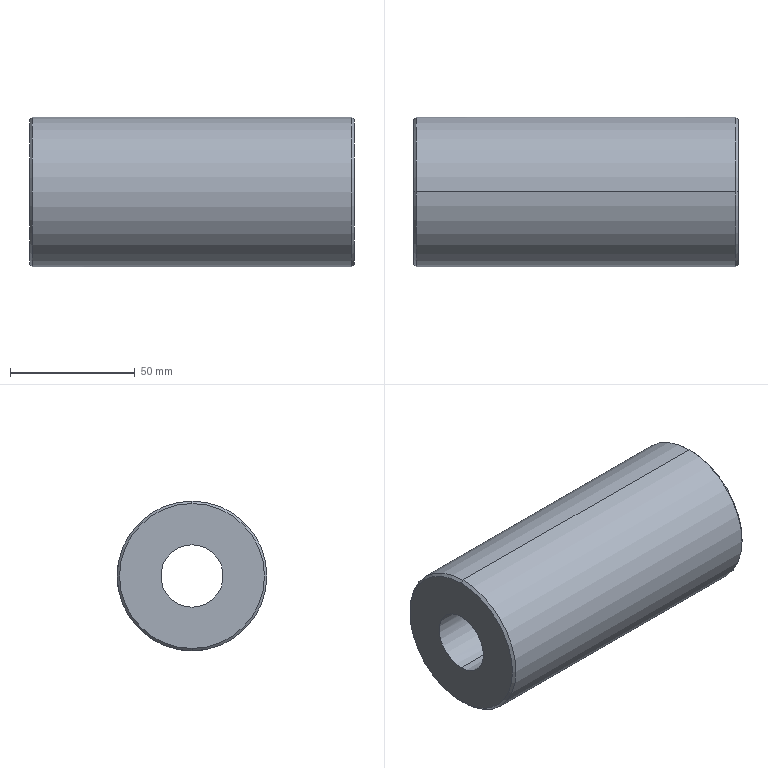Part | STEP file | Sleeve | 1 solid | 18 faces | box 130 x 60 x 60 mm | volume 302189 mm3 | cylinder 12 | cone 4 | plane 2 | commonest cylinder face diameters 5 x8 25 x2 60 x2
STEP:
#1=CARTESIAN_POINT('',(40.,29.896,2.5));
#2=VERTEX_POINT('',#1);
#3=CARTESIAN_POINT('',(40.,29.896,-2.5));
#4=VERTEX_POINT('',#3);
#5=CARTESIAN_POINT('',(40.,29.896,2.5));
#6=CARTESIAN_POINT('',(39.835,29.896,2.5));
#7=CARTESIAN_POINT('',(39.672,29.897,2.484));
#8=CARTESIAN_POINT('',(39.353,29.902,2.42));
#9=CARTESIAN_POINT('',(39.194,29.906,2.372));
#10=CARTESIAN_POINT('',(38.891,29.916,2.247));
#11=CARTESIAN_POINT('',(38.748,29.922,2.17));
#12=CARTESIAN_POINT('',(38.476,29.934,1.989));
#13=CARTESIAN_POINT('',(38.347,29.941,1.883));
#14=CARTESIAN_POINT('',(38.117,29.955,1.652));
#15=CARTESIAN_POINT('',(38.013,29.961,1.527));
#16=CARTESIAN_POINT('',(37.831,29.974,1.253));
#17=CARTESIAN_POINT('',(37.753,29.98,1.108));
#18=CARTESIAN_POINT('',(37.628,29.99,0.8074));
#19=CARTESIAN_POINT('',(37.58,29.993,0.6498));
#20=CARTESIAN_POINT('',(37.516,29.999,0.3271));
#21=CARTESIAN_POINT('',(37.5,30.,0.1648));
#22=CARTESIAN_POINT('',(37.5,30.,-0.1614));
#23=CARTESIAN_POINT('',(37.516,29.999,-0.327));
#24=CARTESIAN_POINT('',(37.58,29.993,-0.6477));
#25=CARTESIAN_POINT('',(37.627,29.99,-0.8036));
#26=CARTESIAN_POINT('',(37.752,29.98,-1.106));
#27=CARTESIAN_POINT('',(37.83,29.974,-1.253));
#28=CARTESIAN_POINT('',(38.011,29.962,-1.524));
#29=CARTESIAN_POINT('',(38.114,29.955,-1.65));
#30=CARTESIAN_POINT('',(38.348,29.941,-1.883));
#31=CARTESIAN_POINT('',(38.474,29.934,-1.987));
#32=CARTESIAN_POINT('',(38.744,29.922,-2.168));
#33=CARTESIAN_POINT('',(38.89,29.916,-2.246));
#34=CARTESIAN_POINT('',(39.193,29.906,-2.372));
#35=CARTESIAN_POINT('',(39.349,29.902,-2.419));
#36=CARTESIAN_POINT('',(39.669,29.897,-2.483));
#37=CARTESIAN_POINT('',(39.835,29.896,-2.5));
#38=CARTESIAN_POINT('',(40.,29.896,-2.5));
#39=B_SPLINE_CURVE_WITH_KNOTS('',3,(#5,#6,#7,#8,#9,#10,#11,#12,#13,#14,#15,#16,#17,#18,#19,#20,#21,#22,#23,#24,#25,#26,#27,#28,#29,#30,#31,#32,#33,#34,#35,#36,#37,#38),.UNSPECIFIED.,.F.,.F.,(4,2,2,2,2,2,2,2,2,2,2,2,2,2,2,2,4),(0.007818,0.008306,0.008795,0.009284,0.009772,0.01026,0.01075,0.01124,0.01173,0.01222,0.0127,0.01319,0.01368,0.01417,0.01466,0.01515,0.01564),.UNSPECIFIED.);
#40=EDGE_CURVE('',#2,#4,#39,.T.);
#41=ORIENTED_EDGE('',*,*,#40,.T.);
#42=CARTESIAN_POINT('',(40.,29.896,-2.5));
#43=CARTESIAN_POINT('',(40.165,29.896,-2.5));
#44=CARTESIAN_POINT('',(40.328,29.897,-2.484));
#45=CARTESIAN_POINT('',(40.647,29.902,-2.42));
#46=CARTESIAN_POINT('',(40.806,29.906,-2.372));
#47=CARTESIAN_POINT('',(41.109,29.916,-2.247));
#48=CARTESIAN_POINT('',(41.252,29.922,-2.17));
#49=CARTESIAN_POINT('',(41.524,29.934,-1.989));
#50=CARTESIAN_POINT('',(41.653,29.941,-1.883));
#51=CARTESIAN_POINT('',(41.883,29.955,-1.652));
#52=CARTESIAN_POINT('',(41.987,29.961,-1.527));
#53=CARTESIAN_POINT('',(42.169,29.974,-1.253));
#54=CARTESIAN_POINT('',(42.247,29.98,-1.108));
#55=CARTESIAN_POINT('',(42.372,29.99,-0.8074));
#56=CARTESIAN_POINT('',(42.42,29.993,-0.6498));
#57=CARTESIAN_POINT('',(42.484,29.999,-0.3271));
#58=CARTESIAN_POINT('',(42.5,30.,-0.1648));
#59=CARTESIAN_POINT('',(42.5,30.,0.1614));
#60=CARTESIAN_POINT('',(42.484,29.999,0.327));
#61=CARTESIAN_POINT('',(42.42,29.993,0.6477));
#62=CARTESIAN_POINT('',(42.373,29.99,0.8036));
#63=CARTESIAN_POINT('',(42.248,29.98,1.106));
#64=CARTESIAN_POINT('',(42.17,29.974,1.253));
#65=CARTESIAN_POINT('',(41.989,29.962,1.524));
#66=CARTESIAN_POINT('',(41.886,29.955,1.65));
#67=CARTESIAN_POINT('',(41.652,29.941,1.883));
#68=CARTESIAN_POINT('',(41.526,29.934,1.987));
#69=CARTESIAN_POINT('',(41.256,29.922,2.168));
#70=CARTESIAN_POINT('',(41.11,29.916,2.246));
#71=CARTESIAN_POINT('',(40.807,29.906,2.372));
#72=CARTESIAN_POINT('',(40.651,29.902,2.419));
#73=CARTESIAN_POINT('',(40.331,29.897,2.483));
#74=CARTESIAN_POINT('',(40.165,29.896,2.5));
#75=CARTESIAN_POINT('',(40.,29.896,2.5));
#76=B_SPLINE_CURVE_WITH_KNOTS('',3,(#42,#43,#44,#45,#46,#47,#48,#49,#50,#51,#52,#53,#54,#55,#56,#57,#58,#59,#60,#61,#62,#63,#64,#65,#66,#67,#68,#69,#70,#71,#72,#73,#74,#75),.UNSPECIFIED.,.F.,.F.,(4,2,2,2,2,2,2,2,2,2,2,2,2,2,2,2,4),(0.,0.0004886,0.0009772,0.001466,0.001954,0.002443,0.002932,0.00342,0.003909,0.004398,0.004886,0.005375,0.005863,0.006352,0.006841,0.007329,0.007818),.UNSPECIFIED.);
#77=EDGE_CURVE('',#4,#2,#76,.T.);
#78=ORIENTED_EDGE('',*,*,#77,.T.);
#79=EDGE_LOOP('',(#41,#78));
#80=FACE_BOUND('',#79,.T.);
#81=CARTESIAN_POINT('',(-40.,29.896,2.5));
#82=VERTEX_POINT('',#81);
#83=CARTESIAN_POINT('',(-40.,29.896,-2.5));
#84=VERTEX_POINT('',#83);
#85=CARTESIAN_POINT('',(-40.,29.896,2.5));
#86=CARTESIAN_POINT('',(-40.165,29.896,2.5));
#87=CARTESIAN_POINT('',(-40.328,29.897,2.484));
#88=CARTESIAN_POINT('',(-40.647,29.902,2.42));
#89=CARTESIAN_POINT('',(-40.806,29.906,2.372));
#90=CARTESIAN_POINT('',(-41.109,29.916,2.247));
#91=CARTESIAN_POINT('',(-41.252,29.922,2.17));
#92=CARTESIAN_POINT('',(-41.524,29.934,1.989));
#93=CARTESIAN_POINT('',(-41.653,29.941,1.883));
#94=CARTESIAN_POINT('',(-41.883,29.955,1.652));
#95=CARTESIAN_POINT('',(-41.987,29.961,1.527));
#96=CARTESIAN_POINT('',(-42.169,29.974,1.253));
#97=CARTESIAN_POINT('',(-42.247,29.98,1.108));
#98=CARTESIAN_POINT('',(-42.372,29.99,0.8074));
#99=CARTESIAN_POINT('',(-42.42,29.993,0.6498));
#100=CARTESIAN_POINT('',(-42.484,29.999,0.3271));
#101=CARTESIAN_POINT('',(-42.5,30.,0.1648));
#102=CARTESIAN_POINT('',(-42.5,30.,-0.1614));
#103=CARTESIAN_POINT('',(-42.484,29.999,-0.327));
#104=CARTESIAN_POINT('',(-42.42,29.993,-0.6477));
#105=CARTESIAN_POINT('',(-42.373,29.99,-0.8036));
#106=CARTESIAN_POINT('',(-42.248,29.98,-1.106));
#107=CARTESIAN_POINT('',(-42.17,29.974,-1.253));
#108=CARTESIAN_POINT('',(-41.989,29.962,-1.524));
#109=CARTESIAN_POINT('',(-41.886,29.955,-1.65));
#110=CARTESIAN_POINT('',(-41.652,29.941,-1.883));
#111=CARTESIAN_POINT('',(-41.526,29.934,-1.987));
#112=CARTESIAN_POINT('',(-41.256,29.922,-2.168));
#113=CARTESIAN_POINT('',(-41.11,29.916,-2.246));
#114=CARTESIAN_POINT('',(-40.807,29.906,-2.372));
#115=CARTESIAN_POINT('',(-40.651,29.902,-2.419));
#116=CARTESIAN_POINT('',(-40.331,29.897,-2.483));
#117=CARTESIAN_POINT('',(-40.165,29.896,-2.5));
#118=CARTESIAN_POINT('',(-40.,29.896,-2.5));
#119=B_SPLINE_CURVE_WITH_KNOTS('',3,(#85,#86,#87,#88,#89,#90,#91,#92,#93,#94,#95,#96,#97,#98,#99,#100,#101,#102,#103,#104,#105,#106,#107,#108,#109,#110,#111,#112,#113,#114,#115,#116,#117,#118),.UNSPECIFIED.,.F.,.F.,(4,2,2,2,2,2,2,2,2,2,2,2,2,2,2,2,4),(0.007818,0.008306,0.008795,0.009284,0.009772,0.01026,0.01075,0.01124,0.01173,0.01222,0.0127,0.01319,0.01368,0.01417,0.01466,0.01515,0.01564),.UNSPECIFIED.);
#120=EDGE_CURVE('',#82,#84,#119,.T.);
#121=ORIENTED_EDGE('',*,*,#120,.T.);
#122=CARTESIAN_POINT('',(-40.,29.896,-2.5));
#123=CARTESIAN_POINT('',(-39.835,29.896,-2.5));
#124=CARTESIAN_POINT('',(-39.672,29.897,-2.484));
#125=CARTESIAN_POINT('',(-39.353,29.902,-2.42));
#126=CARTESIAN_POINT('',(-39.194,29.906,-2.372));
#127=CARTESIAN_POINT('',(-38.891,29.916,-2.247));
#128=CARTESIAN_POINT('',(-38.748,29.922,-2.17));
#129=CARTESIAN_POINT('',(-38.476,29.934,-1.989));
#130=CARTESIAN_POINT('',(-38.347,29.941,-1.883));
#131=CARTESIAN_POINT('',(-38.117,29.955,-1.652));
#132=CARTESIAN_POINT('',(-38.013,29.961,-1.527));
#133=CARTESIAN_POINT('',(-37.831,29.974,-1.253));
#134=CARTESIAN_POINT('',(-37.753,29.98,-1.108));
#135=CARTESIAN_POINT('',(-37.628,29.99,-0.8074));
#136=CARTESIAN_POINT('',(-37.58,29.993,-0.6498));
#137=CARTESIAN_POINT('',(-37.516,29.999,-0.3271));
#138=CARTESIAN_POINT('',(-37.5,30.,-0.1648));
#139=CARTESIAN_POINT('',(-37.5,30.,0.1614));
#140=CARTESIAN_POINT('',(-37.516,29.999,0.327));
#141=CARTESIAN_POINT('',(-37.58,29.993,0.6477));
#142=CARTESIAN_POINT('',(-37.627,29.99,0.8036));
#143=CARTESIAN_POINT('',(-37.752,29.98,1.106));
#144=CARTESIAN_POINT('',(-37.83,29.974,1.253));
#145=CARTESIAN_POINT('',(-38.011,29.962,1.524));
#146=CARTESIAN_POINT('',(-38.114,29.955,1.65));
#147=CARTESIAN_POINT('',(-38.348,29.941,1.883));
#148=CARTESIAN_POINT('',(-38.474,29.934,1.987));
#149=CARTESIAN_POINT('',(-38.744,29.922,2.168));
#150=CARTESIAN_POINT('',(-38.89,29.916,2.246));
#151=CARTESIAN_POINT('',(-39.193,29.906,2.372));
#152=CARTESIAN_POINT('',(-39.349,29.902,2.419));
#153=CARTESIAN_POINT('',(-39.669,29.897,2.483));
#154=CARTESIAN_POINT('',(-39.835,29.896,2.5));
#155=CARTESIAN_POINT('',(-40.,29.896,2.5));
#156=B_SPLINE_CURVE_WITH_KNOTS('',3,(#122,#123,#124,#125,#126,#127,#128,#129,#130,#131,#132,#133,#134,#135,#136,#137,#138,#139,#140,#141,#142,#143,#144,#145,#146,#147,#148,#149,#150,#151,#152,#153,#154,#155),.UNSPECIFIED.,.F.,.F.,(4,2,2,2,2,2,2,2,2,2,2,2,2,2,2,2,4),(0.,0.0004886,0.0009772,0.001466,0.001954,0.002443,0.002932,0.00342,0.003909,0.004398,0.004886,0.005375,0.005863,0.006352,0.006841,0.007329,0.007818),.UNSPECIFIED.);
#157=EDGE_CURVE('',#84,#82,#156,.T.);
#158=ORIENTED_EDGE('',*,*,#157,.T.);
#159=EDGE_LOOP('',(#121,#158));
#160=FACE_BOUND('',#159,.T.);
#161=CARTESIAN_POINT('',(64.,0.,30.));
#162=VERTEX_POINT('',#161);
#163=CARTESIAN_POINT('',(64.,0.,-30.));
#164=VERTEX_POINT('',#163);
#165=CARTESIAN_POINT('',(64.,0.,0.));
#166=DIRECTION('',(-1.,0.,0.));
#167=DIRECTION('',(0.,0.,1.));
#168=AXIS2_PLACEMENT_3D('',#165,#166,#167);
#169=CIRCLE('',#168,30.);
#170=EDGE_CURVE('',#162,#164,#169,.T.);
#171=ORIENTED_EDGE('',*,*,#170,.T.);
#172=CARTESIAN_POINT('',(42.5,0.,-30.));
#173=VERTEX_POINT('',#172);
#174=CARTESIAN_POINT('',(65.,0.,-30.));
#175=DIRECTION('',(-1.,0.,0.));
#176=VECTOR('',#175,1000.);
#177=LINE('',#174,#176);
#178=EDGE_CURVE('',#164,#173,#177,.T.);
#179=ORIENTED_EDGE('',*,*,#178,.T.);
#180=CARTESIAN_POINT('',(40.,2.5,-29.896));
#181=VERTEX_POINT('',#180);
#182=CARTESIAN_POINT('',(42.5,0.,-30.));
#183=CARTESIAN_POINT('',(42.5,0.1651,-30.));
#184=CARTESIAN_POINT('',(42.484,0.3275,-29.999));
#185=CARTESIAN_POINT('',(42.42,0.6469,-29.993));
#186=CARTESIAN_POINT('',(42.372,0.8057,-29.99));
#187=CARTESIAN_POINT('',(42.247,1.108,-29.98));
#188=CARTESIAN_POINT('',(42.17,1.252,-29.974));
#189=CARTESIAN_POINT('',(41.989,1.523,-29.962));
#190=CARTESIAN_POINT('',(41.884,1.652,-29.955));
#191=CARTESIAN_POINT('',(41.653,1.882,-29.941));
#192=CARTESIAN_POINT('',(41.528,1.986,-29.934));
#193=CARTESIAN_POINT('',(41.255,2.169,-29.922));
#194=CARTESIAN_POINT('',(41.109,2.246,-29.916));
#195=CARTESIAN_POINT('',(40.658,2.434,-29.901));
#196=CARTESIAN_POINT('',(40.33,2.5,-29.896));
#197=CARTESIAN_POINT('',(40.,2.5,-29.896));
#198=B_SPLINE_CURVE_WITH_KNOTS('',3,(#182,#183,#184,#185,#186,#187,#188,#189,#190,#191,#192,#193,#194,#195,#196,#197),.UNSPECIFIED.,.F.,.F.,(4,2,2,2,2,2,2,4),(0.007814,0.008303,0.008791,0.009279,0.009768,0.01026,0.01074,0.01172),.UNSPECIFIED.);
#199=EDGE_CURVE('',#173,#181,#198,.T.);
#200=ORIENTED_EDGE('',*,*,#199,.T.);
#201=CARTESIAN_POINT('',(37.5,0.,-30.));
#202=VERTEX_POINT('',#201);
#203=CARTESIAN_POINT('',(40.,2.5,-29.896));
#204=CARTESIAN_POINT('',(39.835,2.5,-29.896));
#205=CARTESIAN_POINT('',(39.672,2.484,-29.897));
#206=CARTESIAN_POINT('',(39.353,2.42,-29.902));
#207=CARTESIAN_POINT('',(39.194,2.372,-29.906));
#208=CARTESIAN_POINT('',(38.892,2.247,-29.916));
#209=CARTESIAN_POINT('',(38.748,2.17,-29.922));
#210=CARTESIAN_POINT('',(38.477,1.989,-29.934));
#211=CARTESIAN_POINT('',(38.348,1.884,-29.941));
#212=CARTESIAN_POINT('',(38.118,1.653,-29.955));
#213=CARTESIAN_POINT('',(38.014,1.528,-29.961));
#214=CARTESIAN_POINT('',(37.831,1.255,-29.974));
#215=CARTESIAN_POINT('',(37.754,1.109,-29.98));
#216=CARTESIAN_POINT('',(37.566,0.6585,-29.994));
#217=CARTESIAN_POINT('',(37.5,0.3303,-30.));
#218=CARTESIAN_POINT('',(37.5,0.,-30.));
#219=B_SPLINE_CURVE_WITH_KNOTS('',3,(#203,#204,#205,#206,#207,#208,#209,#210,#211,#212,#213,#214,#215,#216,#217,#218),.UNSPECIFIED.,.F.,.F.,(4,2,2,2,2,2,2,4),(-0.003907,-0.003419,-0.00293,-0.002442,-0.001954,-0.001465,-0.0009768,0.),.UNSPECIFIED.);
#220=EDGE_CURVE('',#181,#202,#219,.T.);
#221=ORIENTED_EDGE('',*,*,#220,.T.);
#222=CARTESIAN_POINT('',(-37.5,0.,-30.));
#223=VERTEX_POINT('',#222);
#224=CARTESIAN_POINT('',(65.,0.,-30.));
#225=DIRECTION('',(-1.,0.,0.));
#226=VECTOR('',#225,1000.);
#227=LINE('',#224,#226);
#228=EDGE_CURVE('',#202,#223,#227,.T.);
#229=ORIENTED_EDGE('',*,*,#228,.T.);
#230=CARTESIAN_POINT('',(-40.,2.5,-29.896));
#231=VERTEX_POINT('',#230);
#232=CARTESIAN_POINT('',(-37.5,0.,-30.));
#233=CARTESIAN_POINT('',(-37.5,0.1651,-30.));
#234=CARTESIAN_POINT('',(-37.516,0.3275,-29.999));
#235=CARTESIAN_POINT('',(-37.58,0.6469,-29.993));
#236=CARTESIAN_POINT('',(-37.628,0.8057,-29.99));
#237=CARTESIAN_POINT('',(-37.753,1.108,-29.98));
#238=CARTESIAN_POINT('',(-37.83,1.252,-29.974));
#239=CARTESIAN_POINT('',(-38.011,1.523,-29.962));
#240=CARTESIAN_POINT('',(-38.116,1.652,-29.955));
#241=CARTESIAN_POINT('',(-38.347,1.882,-29.941));
#242=CARTESIAN_POINT('',(-38.472,1.986,-29.934));
#243=CARTESIAN_POINT('',(-38.745,2.169,-29.922));
#244=CARTESIAN_POINT('',(-38.891,2.246,-29.916));
#245=CARTESIAN_POINT('',(-39.342,2.434,-29.901));
#246=CARTESIAN_POINT('',(-39.67,2.5,-29.896));
#247=CARTESIAN_POINT('',(-40.,2.5,-29.896));
#248=B_SPLINE_CURVE_WITH_KNOTS('',3,(#232,#233,#234,#235,#236,#237,#238,#239,#240,#241,#242,#243,#244,#245,#246,#247),.UNSPECIFIED.,.F.,.F.,(4,2,2,2,2,2,2,4),(0.007814,0.008303,0.008791,0.009279,0.009768,0.01026,0.01074,0.01172),.UNSPECIFIED.);
#249=EDGE_CURVE('',#223,#231,#248,.T.);
#250=ORIENTED_EDGE('',*,*,#249,.T.);
#251=CARTESIAN_POINT('',(-42.5,0.,-30.));
#252=VERTEX_POINT('',#251);
#253=CARTESIAN_POINT('',(-40.,2.5,-29.896));
#254=CARTESIAN_POINT('',(-40.165,2.5,-29.896));
#255=CARTESIAN_POINT('',(-40.328,2.484,-29.897));
#256=CARTESIAN_POINT('',(-40.647,2.42,-29.902));
#257=CARTESIAN_POINT('',(-40.806,2.372,-29.906));
#258=CARTESIAN_POINT('',(-41.108,2.247,-29.916));
#259=CARTESIAN_POINT('',(-41.252,2.17,-29.922));
#260=CARTESIAN_POINT('',(-41.523,1.989,-29.934));
#261=CARTESIAN_POINT('',(-41.652,1.884,-29.941));
#262=CARTESIAN_POINT('',(-41.882,1.653,-29.955));
#263=CARTESIAN_POINT('',(-41.986,1.528,-29.961));
#264=CARTESIAN_POINT('',(-42.169,1.255,-29.974));
#265=CARTESIAN_POINT('',(-42.246,1.109,-29.98));
#266=CARTESIAN_POINT('',(-42.434,0.6585,-29.994));
#267=CARTESIAN_POINT('',(-42.5,0.3303,-30.));
#268=CARTESIAN_POINT('',(-42.5,0.,-30.));
#269=B_SPLINE_CURVE_WITH_KNOTS('',3,(#253,#254,#255,#256,#257,#258,#259,#260,#261,#262,#263,#264,#265,#266,#267,#268),.UNSPECIFIED.,.F.,.F.,(4,2,2,2,2,2,2,4),(0.01172,0.01221,0.0127,0.01319,0.01367,0.01416,0.01465,0.01563),.UNSPECIFIED.);
#270=EDGE_CURVE('',#231,#252,#269,.T.);
#271=ORIENTED_EDGE('',*,*,#270,.T.);
#272=CARTESIAN_POINT('',(-64.,0.,-30.));
#273=VERTEX_POINT('',#272);
#274=CARTESIAN_POINT('',(65.,0.,-30.));
#275=DIRECTION('',(-1.,0.,0.));
#276=VECTOR('',#275,1000.);
#277=LINE('',#274,#276);
#278=EDGE_CURVE('',#252,#273,#277,.T.);
#279=ORIENTED_EDGE('',*,*,#278,.T.);
#280=CARTESIAN_POINT('',(-64.,0.,30.));
#281=VERTEX_POINT('',#280);
#282=CARTESIAN_POINT('',(-64.,0.,0.));
#283=DIRECTION('',(1.,0.,0.));
#284=DIRECTION('',(0.,0.,1.));
#285=AXIS2_PLACEMENT_3D('',#282,#283,#284);
#286=CIRCLE('',#285,30.);
#287=EDGE_CURVE('',#273,#281,#286,.T.);
#288=ORIENTED_EDGE('',*,*,#287,.T.);
#289=CARTESIAN_POINT('',(65.,0.,30.));
#290=DIRECTION('',(-1.,0.,0.));
#291=VECTOR('',#290,1000.);
#292=LINE('',#289,#291);
#293=EDGE_CURVE('',#162,#281,#292,.T.);
#294=ORIENTED_EDGE('',*,*,#293,.F.);
#295=EDGE_LOOP('',(#171,#179,#200,#221,#229,#250,#271,#279,#288,#294));
#296=FACE_OUTER_BOUND('',#295,.T.);
#297=CARTESIAN_POINT('',(65.,0.,0.));
#298=DIRECTION('',(-1.,0.,0.));
#299=DIRECTION('',(0.,0.,1.));
#300=AXIS2_PLACEMENT_3D('',#297,#298,#299);
#301=CYLINDRICAL_SURFACE('',#300,30.);
#302=ADVANCED_FACE('',(#80,#160,#296),#301,.T.);
#303=CARTESIAN_POINT('',(40.,-2.5,-12.247));
#304=VERTEX_POINT('',#303);
#305=CARTESIAN_POINT('',(37.5,0.,-12.5));
#306=VERTEX_POINT('',#305);
#307=CARTESIAN_POINT('',(40.,-2.5,-12.247));
#308=CARTESIAN_POINT('',(39.834,-2.5,-12.247));
#309=CARTESIAN_POINT('',(39.672,-2.484,-12.251));
#310=CARTESIAN_POINT('',(39.352,-2.42,-12.264));
#311=CARTESIAN_POINT('',(39.193,-2.372,-12.273));
#312=CARTESIAN_POINT('',(38.891,-2.246,-12.297));
#313=CARTESIAN_POINT('',(38.747,-2.17,-12.311));
#314=CARTESIAN_POINT('',(38.476,-1.988,-12.341));
#315=CARTESIAN_POINT('',(38.348,-1.883,-12.358));
#316=CARTESIAN_POINT('',(38.003,-1.539,-12.407));
#317=CARTESIAN_POINT('',(37.817,-1.261,-12.44));
#318=CARTESIAN_POINT('',(37.567,-0.6598,-12.486));
#319=CARTESIAN_POINT('',(37.5,-0.331,-12.5));
#320=CARTESIAN_POINT('',(37.5,0.,-12.5));
#321=B_SPLINE_CURVE_WITH_KNOTS('',3,(#307,#308,#309,#310,#311,#312,#313,#314,#315,#316,#317,#318,#319,#320),.UNSPECIFIED.,.F.,.F.,(4,2,2,2,2,2,4),(0.003915,0.004405,0.004894,0.005384,0.005873,0.006852,0.007831),.UNSPECIFIED.);
#322=EDGE_CURVE('',#304,#306,#321,.T.);
#323=ORIENTED_EDGE('',*,*,#322,.F.);
#324=CARTESIAN_POINT('',(40.,-2.5,-29.896));
#325=VERTEX_POINT('',#324);
#326=CARTESIAN_POINT('',(40.,-2.5,-30.));
#327=DIRECTION('',(0.,0.,-1.));
#328=VECTOR('',#327,1000.);
#329=LINE('',#326,#328);
#330=EDGE_CURVE('',#304,#325,#329,.T.);
#331=ORIENTED_EDGE('',*,*,#330,.T.);
#332=CARTESIAN_POINT('',(37.5,0.,-30.));
#333=CARTESIAN_POINT('',(37.5,-0.1651,-30.));
#334=CARTESIAN_POINT('',(37.516,-0.3275,-29.999));
#335=CARTESIAN_POINT('',(37.58,-0.6469,-29.993));
#336=CARTESIAN_POINT('',(37.628,-0.8057,-29.99));
#337=CARTESIAN_POINT('',(37.753,-1.108,-29.98));
#338=CARTESIAN_POINT('',(37.83,-1.252,-29.974));
#339=CARTESIAN_POINT('',(38.011,-1.523,-29.962));
#340=CARTESIAN_POINT('',(38.116,-1.652,-29.955));
#341=CARTESIAN_POINT('',(38.347,-1.882,-29.941));
#342=CARTESIAN_POINT('',(38.472,-1.986,-29.934));
#343=CARTESIAN_POINT('',(38.745,-2.169,-29.922));
#344=CARTESIAN_POINT('',(38.891,-2.246,-29.916));
#345=CARTESIAN_POINT('',(39.342,-2.434,-29.901));
#346=CARTESIAN_POINT('',(39.67,-2.5,-29.896));
#347=CARTESIAN_POINT('',(40.,-2.5,-29.896));
#348=B_SPLINE_CURVE_WITH_KNOTS('',3,(#332,#333,#334,#335,#336,#337,#338,#339,#340,#341,#342,#343,#344,#345,#346,#347),.UNSPECIFIED.,.F.,.F.,(4,2,2,2,2,2,2,4),(0.,0.0004884,0.0009768,0.001465,0.001954,0.002442,0.00293,0.003907),.UNSPECIFIED.);
#349=EDGE_CURVE('',#202,#325,#348,.T.);
#350=ORIENTED_EDGE('',*,*,#349,.F.);
#351=ORIENTED_EDGE('',*,*,#220,.F.);
#352=CARTESIAN_POINT('',(40.,2.5,-12.247));
#353=VERTEX_POINT('',#352);
#354=CARTESIAN_POINT('',(40.,2.5,-30.));
#355=DIRECTION('',(0.,0.,-1.));
#356=VECTOR('',#355,1000.);
#357=LINE('',#354,#356);
#358=EDGE_CURVE('',#353,#181,#357,.T.);
#359=ORIENTED_EDGE('',*,*,#358,.F.);
#360=CARTESIAN_POINT('',(37.5,0.,-12.5));
#361=CARTESIAN_POINT('',(37.5,0.1655,-12.5));
#362=CARTESIAN_POINT('',(37.516,0.3282,-12.497));
#363=CARTESIAN_POINT('',(37.58,0.6481,-12.484));
#364=CARTESIAN_POINT('',(37.628,0.807,-12.475));
#365=CARTESIAN_POINT('',(37.754,1.109,-12.452));
#366=CARTESIAN_POINT('',(37.83,1.253,-12.438));
#367=CARTESIAN_POINT('',(38.012,1.524,-12.407));
#368=CARTESIAN_POINT('',(38.117,1.652,-12.391));
#369=CARTESIAN_POINT('',(38.462,1.997,-12.342));
#370=CARTESIAN_POINT('',(38.739,2.183,-12.309));
#371=CARTESIAN_POINT('',(39.34,2.433,-12.262));
#372=CARTESIAN_POINT('',(39.669,2.5,-12.247));
#373=CARTESIAN_POINT('',(40.,2.5,-12.247));
#374=B_SPLINE_CURVE_WITH_KNOTS('',3,(#360,#361,#362,#363,#364,#365,#366,#367,#368,#369,#370,#371,#372,#373),.UNSPECIFIED.,.F.,.F.,(4,2,2,2,2,2,4),(0.007831,0.00832,0.00881,0.009299,0.009788,0.01077,0.01175),.UNSPECIFIED.);
#375=EDGE_CURVE('',#306,#353,#374,.T.);
#376=ORIENTED_EDGE('',*,*,#375,.F.);
#377=EDGE_LOOP('',(#323,#331,#350,#351,#359,#376));
#378=FACE_OUTER_BOUND('',#377,.T.);
#379=CARTESIAN_POINT('',(40.,0.,-30.));
#380=DIRECTION('',(0.,0.,-1.));
#381=DIRECTION('',(0.,1.,0.));
#382=AXIS2_PLACEMENT_3D('',#379,#380,#381);
#383=CYLINDRICAL_SURFACE('',#382,2.5);
#384=ADVANCED_FACE('',(#378),#383,.F.);
#385=CARTESIAN_POINT('',(-40.,-2.5,-12.247));
#386=VERTEX_POINT('',#385);
#387=CARTESIAN_POINT('',(-42.5,0.,-12.5));
#388=VERTEX_POINT('',#387);
#389=CARTESIAN_POINT('',(-40.,-2.5,-12.247));
#390=CARTESIAN_POINT('',(-40.166,-2.5,-12.247));
#391=CARTESIAN_POINT('',(-40.328,-2.484,-12.251));
#392=CARTESIAN_POINT('',(-40.648,-2.42,-12.264));
#393=CARTESIAN_POINT('',(-40.807,-2.372,-12.273));
#394=CARTESIAN_POINT('',(-41.109,-2.246,-12.297));
#395=CARTESIAN_POINT('',(-41.253,-2.17,-12.311));
#396=CARTESIAN_POINT('',(-41.524,-1.988,-12.341));
#397=CARTESIAN_POINT('',(-41.652,-1.883,-12.358));
#398=CARTESIAN_POINT('',(-41.997,-1.539,-12.407));
#399=CARTESIAN_POINT('',(-42.183,-1.261,-12.44));
#400=CARTESIAN_POINT('',(-42.433,-0.6598,-12.486));
#401=CARTESIAN_POINT('',(-42.5,-0.331,-12.5));
#402=CARTESIAN_POINT('',(-42.5,0.,-12.5));
#403=B_SPLINE_CURVE_WITH_KNOTS('',3,(#389,#390,#391,#392,#393,#394,#395,#396,#397,#398,#399,#400,#401,#402),.UNSPECIFIED.,.F.,.F.,(4,2,2,2,2,2,4),(0.003915,0.004405,0.004894,0.005384,0.005873,0.006852,0.007831),.UNSPECIFIED.);
#404=EDGE_CURVE('',#386,#388,#403,.T.);
#405=ORIENTED_EDGE('',*,*,#404,.F.);
#406=CARTESIAN_POINT('',(-40.,-2.5,-29.896));
#407=VERTEX_POINT('',#406);
#408=CARTESIAN_POINT('',(-40.,-2.5,-30.));
#409=DIRECTION('',(0.,0.,-1.));
#410=VECTOR('',#409,1000.);
#411=LINE('',#408,#410);
#412=EDGE_CURVE('',#386,#407,#411,.T.);
#413=ORIENTED_EDGE('',*,*,#412,.T.);
#414=CARTESIAN_POINT('',(-42.5,0.,-30.));
#415=CARTESIAN_POINT('',(-42.5,-0.1651,-30.));
#416=CARTESIAN_POINT('',(-42.484,-0.3275,-29.999));
#417=CARTESIAN_POINT('',(-42.42,-0.6469,-29.993));
#418=CARTESIAN_POINT('',(-42.372,-0.8057,-29.99));
#419=CARTESIAN_POINT('',(-42.247,-1.108,-29.98));
#420=CARTESIAN_POINT('',(-42.17,-1.252,-29.974));
#421=CARTESIAN_POINT('',(-41.989,-1.523,-29.962));
#422=CARTESIAN_POINT('',(-41.884,-1.652,-29.955));
#423=CARTESIAN_POINT('',(-41.653,-1.882,-29.941));
#424=CARTESIAN_POINT('',(-41.528,-1.986,-29.934));
#425=CARTESIAN_POINT('',(-41.255,-2.169,-29.922));
#426=CARTESIAN_POINT('',(-41.109,-2.246,-29.916));
#427=CARTESIAN_POINT('',(-40.658,-2.434,-29.901));
#428=CARTESIAN_POINT('',(-40.33,-2.5,-29.896));
#429=CARTESIAN_POINT('',(-40.,-2.5,-29.896));
#430=B_SPLINE_CURVE_WITH_KNOTS('',3,(#414,#415,#416,#417,#418,#419,#420,#421,#422,#423,#424,#425,#426,#427,#428,#429),.UNSPECIFIED.,.F.,.F.,(4,2,2,2,2,2,2,4),(0.,0.0004884,0.0009768,0.001465,0.001954,0.002442,0.00293,0.003907),.UNSPECIFIED.);
#431=EDGE_CURVE('',#252,#407,#430,.T.);
#432=ORIENTED_EDGE('',*,*,#431,.F.);
#433=ORIENTED_EDGE('',*,*,#270,.F.);
#434=CARTESIAN_POINT('',(-40.,2.5,-12.247));
#435=VERTEX_POINT('',#434);
#436=CARTESIAN_POINT('',(-40.,2.5,-30.));
#437=DIRECTION('',(0.,0.,-1.));
#438=VECTOR('',#437,1000.);
#439=LINE('',#436,#438);
#440=EDGE_CURVE('',#435,#231,#439,.T.);
#441=ORIENTED_EDGE('',*,*,#440,.F.);
#442=CARTESIAN_POINT('',(-42.5,0.,-12.5));
#443=CARTESIAN_POINT('',(-42.5,0.1655,-12.5));
#444=CARTESIAN_POINT('',(-42.484,0.3282,-12.497));
#445=CARTESIAN_POINT('',(-42.42,0.6481,-12.484));
#446=CARTESIAN_POINT('',(-42.372,0.807,-12.475));
#447=CARTESIAN_POINT('',(-42.246,1.109,-12.452));
#448=CARTESIAN_POINT('',(-42.17,1.253,-12.438));
#449=CARTESIAN_POINT('',(-41.988,1.524,-12.407));
#450=CARTESIAN_POINT('',(-41.883,1.652,-12.391));
#451=CARTESIAN_POINT('',(-41.538,1.997,-12.342));
#452=CARTESIAN_POINT('',(-41.261,2.183,-12.309));
#453=CARTESIAN_POINT('',(-40.66,2.433,-12.262));
#454=CARTESIAN_POINT('',(-40.331,2.5,-12.247));
#455=CARTESIAN_POINT('',(-40.,2.5,-12.247));
#456=B_SPLINE_CURVE_WITH_KNOTS('',3,(#442,#443,#444,#445,#446,#447,#448,#449,#450,#451,#452,#453,#454,#455),.UNSPECIFIED.,.F.,.F.,(4,2,2,2,2,2,4),(0.007831,0.00832,0.00881,0.009299,0.009788,0.01077,0.01175),.UNSPECIFIED.);
#457=EDGE_CURVE('',#388,#435,#456,.T.);
#458=ORIENTED_EDGE('',*,*,#457,.F.);
#459=EDGE_LOOP('',(#405,#413,#432,#433,#441,#458));
#460=FACE_OUTER_BOUND('',#459,.T.);
#461=CARTESIAN_POINT('',(-40.,0.,-30.));
#462=DIRECTION('',(0.,0.,-1.));
#463=DIRECTION('',(0.,1.,0.));
#464=AXIS2_PLACEMENT_3D('',#461,#462,#463);
#465=CYLINDRICAL_SURFACE('',#464,2.5);
#466=ADVANCED_FACE('',(#460),#465,.F.);
#467=CARTESIAN_POINT('',(-65.,0.,-29.));
#468=VERTEX_POINT('',#467);
#469=CARTESIAN_POINT('',(-65.,0.,29.));
#470=VERTEX_POINT('',#469);
#471=CARTESIAN_POINT('',(-65.,0.,0.));
#472=DIRECTION('',(1.,0.,0.));
#473=DIRECTION('',(0.,0.,-1.));
#474=AXIS2_PLACEMENT_3D('',#471,#472,#473);
#475=CIRCLE('',#474,29.);
#476=EDGE_CURVE('',#468,#470,#475,.T.);
#477=ORIENTED_EDGE('',*,*,#476,.T.);
#478=CARTESIAN_POINT('',(-64.,0.,30.));
#479=DIRECTION('',(0.7071,0.,0.7071));
#480=VECTOR('',#479,1000.);
#481=LINE('',#478,#480);
#482=EDGE_CURVE('',#470,#281,#481,.T.);
#483=ORIENTED_EDGE('',*,*,#482,.T.);
#484=ORIENTED_EDGE('',*,*,#287,.F.);
#485=CARTESIAN_POINT('',(-64.,0.,-30.));
#486=DIRECTION('',(0.7071,0.,-0.7071));
#487=VECTOR('',#486,1000.);
#488=LINE('',#485,#487);
#489=EDGE_CURVE('',#468,#273,#488,.T.);
#490=ORIENTED_EDGE('',*,*,#489,.F.);
#491=EDGE_LOOP('',(#477,#483,#484,#490));
#492=FACE_OUTER_BOUND('',#491,.T.);
#493=CARTESIAN_POINT('',(-64.,0.,0.));
#494=DIRECTION('',(1.,0.,0.));
#495=DIRECTION('',(0.,0.,-1.));
#496=AXIS2_PLACEMENT_3D('',#493,#494,#495);
#497=CONICAL_SURFACE('',#496,30.,0.7854);
#498=ADVANCED_FACE('',(#492),#497,.T.);
#499=CARTESIAN_POINT('',(65.,0.,29.));
#500=VERTEX_POINT('',#499);
#501=CARTESIAN_POINT('',(65.,0.,-29.));
#502=VERTEX_POINT('',#501);
#503=CARTESIAN_POINT('',(65.,0.,0.));
#504=DIRECTION('',(-1.,0.,0.));
#505=DIRECTION('',(0.,0.,1.));
#506=AXIS2_PLACEMENT_3D('',#503,#504,#505);
#507=CIRCLE('',#506,29.);
#508=EDGE_CURVE('',#500,#502,#507,.T.);
#509=ORIENTED_EDGE('',*,*,#508,.T.);
#510=CARTESIAN_POINT('',(64.,0.,-30.));
#511=DIRECTION('',(-0.7071,0.,-0.7071));
#512=VECTOR('',#511,1000.);
#513=LINE('',#510,#512);
#514=EDGE_CURVE('',#502,#164,#513,.T.);
#515=ORIENTED_EDGE('',*,*,#514,.T.);
#516=ORIENTED_EDGE('',*,*,#170,.F.);
#517=CARTESIAN_POINT('',(64.,0.,30.));
#518=DIRECTION('',(-0.7071,0.,0.7071));
#519=VECTOR('',#518,1000.);
#520=LINE('',#517,#519);
#521=EDGE_CURVE('',#500,#162,#520,.T.);
#522=ORIENTED_EDGE('',*,*,#521,.F.);
#523=EDGE_LOOP('',(#509,#515,#516,#522));
#524=FACE_OUTER_BOUND('',#523,.T.);
#525=CARTESIAN_POINT('',(64.,0.,0.));
#526=DIRECTION('',(-1.,0.,0.));
#527=DIRECTION('',(0.,0.,1.));
#528=AXIS2_PLACEMENT_3D('',#525,#526,#527);
#529=CONICAL_SURFACE('',#528,30.,0.7854);
#530=ADVANCED_FACE('',(#524),#529,.T.);
#531=CARTESIAN_POINT('',(65.,0.,-12.5));
#532=VERTEX_POINT('',#531);
#533=CARTESIAN_POINT('',(65.,0.,12.5));
#534=VERTEX_POINT('',#533);
#535=CARTESIAN_POINT('',(65.,0.,0.));
#536=DIRECTION('',(-1.,0.,0.));
#537=DIRECTION('',(0.,0.,1.));
#538=AXIS2_PLACEMENT_3D('',#535,#536,#537);
#539=CIRCLE('',#538,12.5);
#540=EDGE_CURVE('',#532,#534,#539,.T.);
#541=ORIENTED_EDGE('',*,*,#540,.F.);
#542=CARTESIAN_POINT('',(42.5,0.,-12.5));
#543=VERTEX_POINT('',#542);
#544=CARTESIAN_POINT('',(65.,0.,-12.5));
#545=DIRECTION('',(-1.,0.,0.));
#546=VECTOR('',#545,1000.);
#547=LINE('',#544,#546);
#548=EDGE_CURVE('',#532,#543,#547,.T.);
#549=ORIENTED_EDGE('',*,*,#548,.T.);
#550=CARTESIAN_POINT('',(42.5,0.,-12.5));
#551=CARTESIAN_POINT('',(42.5,-0.1655,-12.5));
#552=CARTESIAN_POINT('',(42.484,-0.3282,-12.497));
#553=CARTESIAN_POINT('',(42.42,-0.6481,-12.484));
#554=CARTESIAN_POINT('',(42.372,-0.807,-12.475));
#555=CARTESIAN_POINT('',(42.246,-1.109,-12.452));
#556=CARTESIAN_POINT('',(42.17,-1.253,-12.438));
#557=CARTESIAN_POINT('',(41.988,-1.524,-12.407));
#558=CARTESIAN_POINT('',(41.883,-1.652,-12.391));
#559=CARTESIAN_POINT('',(41.538,-1.997,-12.342));
#560=CARTESIAN_POINT('',(41.261,-2.183,-12.309));
#561=CARTESIAN_POINT('',(40.66,-2.433,-12.262));
#562=CARTESIAN_POINT('',(40.331,-2.5,-12.247));
#563=CARTESIAN_POINT('',(40.,-2.5,-12.247));
#564=B_SPLINE_CURVE_WITH_KNOTS('',3,(#550,#551,#552,#553,#554,#555,#556,#557,#558,#559,#560,#561,#562,#563),.UNSPECIFIED.,.F.,.F.,(4,2,2,2,2,2,4),(0.,0.0004894,0.0009788,0.001468,0.001958,0.002936,0.003915),.UNSPECIFIED.);
#565=EDGE_CURVE('',#543,#304,#564,.T.);
#566=ORIENTED_EDGE('',*,*,#565,.T.);
#567=ORIENTED_EDGE('',*,*,#322,.T.);
#568=CARTESIAN_POINT('',(-37.5,0.,-12.5));
#569=VERTEX_POINT('',#568);
#570=CARTESIAN_POINT('',(65.,0.,-12.5));
#571=DIRECTION('',(-1.,0.,0.));
#572=VECTOR('',#571,1000.);
#573=LINE('',#570,#572);
#574=EDGE_CURVE('',#306,#569,#573,.T.);
#575=ORIENTED_EDGE('',*,*,#574,.T.);
#576=CARTESIAN_POINT('',(-37.5,0.,-12.5));
#577=CARTESIAN_POINT('',(-37.5,-0.1655,-12.5));
#578=CARTESIAN_POINT('',(-37.516,-0.3282,-12.497));
#579=CARTESIAN_POINT('',(-37.58,-0.6481,-12.484));
#580=CARTESIAN_POINT('',(-37.628,-0.807,-12.475));
#581=CARTESIAN_POINT('',(-37.754,-1.109,-12.452));
#582=CARTESIAN_POINT('',(-37.83,-1.253,-12.438));
#583=CARTESIAN_POINT('',(-38.012,-1.524,-12.407));
#584=CARTESIAN_POINT('',(-38.117,-1.652,-12.391));
#585=CARTESIAN_POINT('',(-38.462,-1.997,-12.342));
#586=CARTESIAN_POINT('',(-38.739,-2.183,-12.309));
#587=CARTESIAN_POINT('',(-39.34,-2.433,-12.262));
#588=CARTESIAN_POINT('',(-39.669,-2.5,-12.247));
#589=CARTESIAN_POINT('',(-40.,-2.5,-12.247));
#590=B_SPLINE_CURVE_WITH_KNOTS('',3,(#576,#577,#578,#579,#580,#581,#582,#583,#584,#585,#586,#587,#588,#589),.UNSPECIFIED.,.F.,.F.,(4,2,2,2,2,2,4),(0.,0.0004894,0.0009788,0.001468,0.001958,0.002936,0.003915),.UNSPECIFIED.);
#591=EDGE_CURVE('',#569,#386,#590,.T.);
#592=ORIENTED_EDGE('',*,*,#591,.T.);
#593=ORIENTED_EDGE('',*,*,#404,.T.);
#594=CARTESIAN_POINT('',(-65.,0.,-12.5));
#595=VERTEX_POINT('',#594);
#596=CARTESIAN_POINT('',(65.,0.,-12.5));
#597=DIRECTION('',(-1.,0.,0.));
#598=VECTOR('',#597,1000.);
#599=LINE('',#596,#598);
#600=EDGE_CURVE('',#388,#595,#599,.T.);
#601=ORIENTED_EDGE('',*,*,#600,.T.);
#602=CARTESIAN_POINT('',(-65.,0.,12.5));
#603=VERTEX_POINT('',#602);
#604=CARTESIAN_POINT('',(-65.,0.,0.));
#605=DIRECTION('',(1.,0.,0.));
#606=DIRECTION('',(0.,0.,1.));
#607=AXIS2_PLACEMENT_3D('',#604,#605,#606);
#608=CIRCLE('',#607,12.5);
#609=EDGE_CURVE('',#603,#595,#608,.T.);
#610=ORIENTED_EDGE('',*,*,#609,.F.);
#611=CARTESIAN_POINT('',(65.,0.,12.5));
#612=DIRECTION('',(-1.,0.,0.));
#613=VECTOR('',#612,1000.);
#614=LINE('',#611,#613);
#615=EDGE_CURVE('',#534,#603,#614,.T.);
#616=ORIENTED_EDGE('',*,*,#615,.F.);
#617=EDGE_LOOP('',(#541,#549,#566,#567,#575,#592,#593,#601,#610,#616));
#618=FACE_OUTER_BOUND('',#617,.T.);
#619=CARTESIAN_POINT('',(65.,0.,0.));
#620=DIRECTION('',(-1.,0.,0.));
#621=DIRECTION('',(0.,0.,1.));
#622=AXIS2_PLACEMENT_3D('',#619,#620,#621);
#623=CYLINDRICAL_SURFACE('',#622,12.5);
#624=ADVANCED_FACE('',(#618),#623,.F.);
#625=CARTESIAN_POINT('',(40.,12.247,2.5));
#626=VERTEX_POINT('',#625);
#627=CARTESIAN_POINT('',(40.,12.247,-2.5));
#628=VERTEX_POINT('',#627);
#629=CARTESIAN_POINT('',(40.,12.247,2.5));
#630=CARTESIAN_POINT('',(39.834,12.247,2.5));
#631=CARTESIAN_POINT('',(39.672,12.251,2.484));
#632=CARTESIAN_POINT('',(39.352,12.264,2.42));
#633=CARTESIAN_POINT('',(39.193,12.273,2.372));
#634=CARTESIAN_POINT('',(38.89,12.297,2.246));
#635=CARTESIAN_POINT('',(38.747,12.311,2.169));
#636=CARTESIAN_POINT('',(38.475,12.341,1.988));
#637=CARTESIAN_POINT('',(38.347,12.358,1.883));
#638=CARTESIAN_POINT('',(38.002,12.407,1.538));
#639=CARTESIAN_POINT('',(37.816,12.44,1.26));
#640=CARTESIAN_POINT('',(37.629,12.475,0.8088));
#641=CARTESIAN_POINT('',(37.581,12.484,0.6508));
#642=CARTESIAN_POINT('',(37.516,12.497,0.328));
#643=CARTESIAN_POINT('',(37.5,12.5,0.1655));
#644=CARTESIAN_POINT('',(37.5,12.5,-0.1614));
#645=CARTESIAN_POINT('',(37.516,12.497,-0.3276));
#646=CARTESIAN_POINT('',(37.58,12.484,-0.6485));
#647=CARTESIAN_POINT('',(37.627,12.475,-0.8045));
#648=CARTESIAN_POINT('',(37.753,12.452,-1.108));
#649=CARTESIAN_POINT('',(37.831,12.438,-1.253));
#650=CARTESIAN_POINT('',(38.011,12.408,-1.524));
#651=CARTESIAN_POINT('',(38.115,12.391,-1.651));
#652=CARTESIAN_POINT('',(38.347,12.358,-1.883));
#653=CARTESIAN_POINT('',(38.473,12.342,-1.986));
#654=CARTESIAN_POINT('',(38.743,12.311,-2.167));
#655=CARTESIAN_POINT('',(38.89,12.297,-2.246));
#656=CARTESIAN_POINT('',(39.192,12.273,-2.371));
#657=CARTESIAN_POINT('',(39.347,12.264,-2.419));
#658=CARTESIAN_POINT('',(39.669,12.251,-2.483));
#659=CARTESIAN_POINT('',(39.834,12.247,-2.5));
#660=CARTESIAN_POINT('',(40.,12.247,-2.5));
#661=B_SPLINE_CURVE_WITH_KNOTS('',3,(#629,#630,#631,#632,#633,#634,#635,#636,#637,#638,#639,#640,#641,#642,#643,#644,#645,#646,#647,#648,#649,#650,#651,#652,#653,#654,#655,#656,#657,#658,#659,#660),.UNSPECIFIED.,.F.,.F.,(4,2,2,2,2,2,2,2,2,2,2,2,2,2,2,4),(0.,0.0004896,0.0009792,0.001469,0.001958,0.002938,0.003427,0.003917,0.004407,0.004896,0.005386,0.005875,0.006365,0.006855,0.007344,0.007834),.UNSPECIFIED.);
#662=EDGE_CURVE('',#626,#628,#661,.T.);
#663=ORIENTED_EDGE('',*,*,#662,.T.);
#664=CARTESIAN_POINT('',(40.,30.,-2.5));
#665=DIRECTION('',(0.,1.,0.));
#666=VECTOR('',#665,1000.);
#667=LINE('',#664,#666);
#668=EDGE_CURVE('',#628,#4,#667,.T.);
#669=ORIENTED_EDGE('',*,*,#668,.T.);
#670=ORIENTED_EDGE('',*,*,#40,.F.);
#671=CARTESIAN_POINT('',(40.,30.,2.5));
#672=DIRECTION('',(0.,1.,0.));
#673=VECTOR('',#672,1000.);
#674=LINE('',#671,#673);
#675=EDGE_CURVE('',#626,#2,#674,.T.);
#676=ORIENTED_EDGE('',*,*,#675,.F.);
#677=EDGE_LOOP('',(#663,#669,#670,#676));
#678=FACE_OUTER_BOUND('',#677,.T.);
#679=CARTESIAN_POINT('',(40.,30.,0.));
#680=DIRECTION('',(0.,1.,0.));
#681=DIRECTION('',(0.,0.,1.));
#682=AXIS2_PLACEMENT_3D('',#679,#680,#681);
#683=CYLINDRICAL_SURFACE('',#682,2.5);
#684=ADVANCED_FACE('',(#678),#683,.F.);
#685=CARTESIAN_POINT('',(-40.,12.247,2.5));
#686=VERTEX_POINT('',#685);
#687=CARTESIAN_POINT('',(-40.,12.247,-2.5));
#688=VERTEX_POINT('',#687);
#689=CARTESIAN_POINT('',(-40.,12.247,2.5));
#690=CARTESIAN_POINT('',(-40.166,12.247,2.5));
#691=CARTESIAN_POINT('',(-40.328,12.251,2.484));
#692=CARTESIAN_POINT('',(-40.648,12.264,2.42));
#693=CARTESIAN_POINT('',(-40.807,12.273,2.372));
#694=CARTESIAN_POINT('',(-41.11,12.297,2.246));
#695=CARTESIAN_POINT('',(-41.253,12.311,2.169));
#696=CARTESIAN_POINT('',(-41.525,12.341,1.988));
#697=CARTESIAN_POINT('',(-41.653,12.358,1.883));
#698=CARTESIAN_POINT('',(-41.998,12.407,1.538));
#699=CARTESIAN_POINT('',(-42.184,12.44,1.26));
#700=CARTESIAN_POINT('',(-42.371,12.475,0.8088));
#701=CARTESIAN_POINT('',(-42.419,12.484,0.6508));
#702=CARTESIAN_POINT('',(-42.484,12.497,0.328));
#703=CARTESIAN_POINT('',(-42.5,12.5,0.1655));
#704=CARTESIAN_POINT('',(-42.5,12.5,-0.1614));
#705=CARTESIAN_POINT('',(-42.484,12.497,-0.3276));
#706=CARTESIAN_POINT('',(-42.42,12.484,-0.6485));
#707=CARTESIAN_POINT('',(-42.373,12.475,-0.8045));
#708=CARTESIAN_POINT('',(-42.247,12.452,-1.108));
#709=CARTESIAN_POINT('',(-42.169,12.438,-1.253));
#710=CARTESIAN_POINT('',(-41.989,12.408,-1.524));
#711=CARTESIAN_POINT('',(-41.885,12.391,-1.651));
#712=CARTESIAN_POINT('',(-41.653,12.358,-1.883));
#713=CARTESIAN_POINT('',(-41.527,12.342,-1.986));
#714=CARTESIAN_POINT('',(-41.257,12.311,-2.167));
#715=CARTESIAN_POINT('',(-41.11,12.297,-2.246));
#716=CARTESIAN_POINT('',(-40.808,12.273,-2.371));
#717=CARTESIAN_POINT('',(-40.653,12.264,-2.419));
#718=CARTESIAN_POINT('',(-40.331,12.251,-2.483));
#719=CARTESIAN_POINT('',(-40.166,12.247,-2.5));
#720=CARTESIAN_POINT('',(-40.,12.247,-2.5));
#721=B_SPLINE_CURVE_WITH_KNOTS('',3,(#689,#690,#691,#692,#693,#694,#695,#696,#697,#698,#699,#700,#701,#702,#703,#704,#705,#706,#707,#708,#709,#710,#711,#712,#713,#714,#715,#716,#717,#718,#719,#720),.UNSPECIFIED.,.F.,.F.,(4,2,2,2,2,2,2,2,2,2,2,2,2,2,2,4),(0.,0.0004896,0.0009792,0.001469,0.001958,0.002938,0.003427,0.003917,0.004407,0.004896,0.005386,0.005875,0.006365,0.006855,0.007344,0.007834),.UNSPECIFIED.);
#722=EDGE_CURVE('',#686,#688,#721,.T.);
#723=ORIENTED_EDGE('',*,*,#722,.T.);
#724=CARTESIAN_POINT('',(-40.,30.,-2.5));
#725=DIRECTION('',(0.,1.,0.));
#726=VECTOR('',#725,1000.);
#727=LINE('',#724,#726);
#728=EDGE_CURVE('',#688,#84,#727,.T.);
#729=ORIENTED_EDGE('',*,*,#728,.T.);
#730=ORIENTED_EDGE('',*,*,#120,.F.);
#731=CARTESIAN_POINT('',(-40.,30.,2.5));
#732=DIRECTION('',(0.,1.,0.));
#733=VECTOR('',#732,1000.);
#734=LINE('',#731,#733);
#735=EDGE_CURVE('',#686,#82,#734,.T.);
#736=ORIENTED_EDGE('',*,*,#735,.F.);
#737=EDGE_LOOP('',(#723,#729,#730,#736));
#738=FACE_OUTER_BOUND('',#737,.T.);
#739=CARTESIAN_POINT('',(-40.,30.,0.));
#740=DIRECTION('',(0.,1.,0.));
#741=DIRECTION('',(0.,0.,1.));
#742=AXIS2_PLACEMENT_3D('',#739,#740,#741);
#743=CYLINDRICAL_SURFACE('',#742,2.5);
#744=ADVANCED_FACE('',(#738),#743,.F.);
#745=ORIENTED_EDGE('',*,*,#178,.F.);
#746=CARTESIAN_POINT('',(64.,0.,0.));
#747=DIRECTION('',(-1.,0.,0.));
#748=DIRECTION('',(0.,0.,1.));
#749=AXIS2_PLACEMENT_3D('',#746,#747,#748);
#750=CIRCLE('',#749,30.);
#751=EDGE_CURVE('',#164,#162,#750,.T.);
#752=ORIENTED_EDGE('',*,*,#751,.T.);
#753=ORIENTED_EDGE('',*,*,#293,.T.);
#754=CARTESIAN_POINT('',(-64.,0.,0.));
#755=DIRECTION('',(1.,0.,0.));
#756=DIRECTION('',(0.,0.,1.));
#757=AXIS2_PLACEMENT_3D('',#754,#755,#756);
#758=CIRCLE('',#757,30.);
#759=EDGE_CURVE('',#281,#273,#758,.T.);
#760=ORIENTED_EDGE('',*,*,#759,.T.);
#761=ORIENTED_EDGE('',*,*,#278,.F.);
#762=ORIENTED_EDGE('',*,*,#431,.T.);
#763=CARTESIAN_POINT('',(-40.,-2.5,-29.896));
#764=CARTESIAN_POINT('',(-39.835,-2.5,-29.896));
#765=CARTESIAN_POINT('',(-39.672,-2.484,-29.897));
#766=CARTESIAN_POINT('',(-39.353,-2.42,-29.902));
#767=CARTESIAN_POINT('',(-39.194,-2.372,-29.906));
#768=CARTESIAN_POINT('',(-38.892,-2.247,-29.916));
#769=CARTESIAN_POINT('',(-38.748,-2.17,-29.922));
#770=CARTESIAN_POINT('',(-38.477,-1.989,-29.934));
#771=CARTESIAN_POINT('',(-38.348,-1.884,-29.941));
#772=CARTESIAN_POINT('',(-38.118,-1.653,-29.955));
#773=CARTESIAN_POINT('',(-38.014,-1.528,-29.961));
#774=CARTESIAN_POINT('',(-37.831,-1.255,-29.974));
#775=CARTESIAN_POINT('',(-37.754,-1.109,-29.98));
#776=CARTESIAN_POINT('',(-37.566,-0.6585,-29.994));
#777=CARTESIAN_POINT('',(-37.5,-0.3303,-30.));
#778=CARTESIAN_POINT('',(-37.5,0.,-30.));
#779=B_SPLINE_CURVE_WITH_KNOTS('',3,(#763,#764,#765,#766,#767,#768,#769,#770,#771,#772,#773,#774,#775,#776,#777,#778),.UNSPECIFIED.,.F.,.F.,(4,2,2,2,2,2,2,4),(0.003907,0.004395,0.004884,0.005372,0.005861,0.006349,0.006837,0.007814),.UNSPECIFIED.);
#780=EDGE_CURVE('',#407,#223,#779,.T.);
#781=ORIENTED_EDGE('',*,*,#780,.T.);
#782=ORIENTED_EDGE('',*,*,#228,.F.);
#783=ORIENTED_EDGE('',*,*,#349,.T.);
#784=CARTESIAN_POINT('',(40.,-2.5,-29.896));
#785=CARTESIAN_POINT('',(40.165,-2.5,-29.896));
#786=CARTESIAN_POINT('',(40.328,-2.484,-29.897));
#787=CARTESIAN_POINT('',(40.647,-2.42,-29.902));
#788=CARTESIAN_POINT('',(40.806,-2.372,-29.906));
#789=CARTESIAN_POINT('',(41.108,-2.247,-29.916));
#790=CARTESIAN_POINT('',(41.252,-2.17,-29.922));
#791=CARTESIAN_POINT('',(41.523,-1.989,-29.934));
#792=CARTESIAN_POINT('',(41.652,-1.884,-29.941));
#793=CARTESIAN_POINT('',(41.882,-1.653,-29.955));
#794=CARTESIAN_POINT('',(41.986,-1.528,-29.961));
#795=CARTESIAN_POINT('',(42.169,-1.255,-29.974));
#796=CARTESIAN_POINT('',(42.246,-1.109,-29.98));
#797=CARTESIAN_POINT('',(42.434,-0.6585,-29.994));
#798=CARTESIAN_POINT('',(42.5,-0.3303,-30.));
#799=CARTESIAN_POINT('',(42.5,0.,-30.));
#800=B_SPLINE_CURVE_WITH_KNOTS('',3,(#784,#785,#786,#787,#788,#789,#790,#791,#792,#793,#794,#795,#796,#797,#798,#799),.UNSPECIFIED.,.F.,.F.,(4,2,2,2,2,2,2,4),(0.003907,0.004395,0.004884,0.005372,0.005861,0.006349,0.006837,0.007814),.UNSPECIFIED.);
#801=EDGE_CURVE('',#325,#173,#800,.T.);
#802=ORIENTED_EDGE('',*,*,#801,.T.);
#803=EDGE_LOOP('',(#745,#752,#753,#760,#761,#762,#781,#782,#783,#802));
#804=FACE_OUTER_BOUND('',#803,.T.);
#805=CARTESIAN_POINT('',(65.,0.,0.));
#806=DIRECTION('',(-1.,0.,0.));
#807=DIRECTION('',(0.,0.,1.));
#808=AXIS2_PLACEMENT_3D('',#805,#806,#807);
#809=CYLINDRICAL_SURFACE('',#808,30.);
#810=ADVANCED_FACE('',(#804),#809,.T.);
#811=ORIENTED_EDGE('',*,*,#330,.F.);
#812=ORIENTED_EDGE('',*,*,#565,.F.);
#813=CARTESIAN_POINT('',(40.,2.5,-12.247));
#814=CARTESIAN_POINT('',(40.166,2.5,-12.247));
#815=CARTESIAN_POINT('',(40.328,2.484,-12.251));
#816=CARTESIAN_POINT('',(40.648,2.42,-12.264));
#817=CARTESIAN_POINT('',(40.807,2.372,-12.273));
#818=CARTESIAN_POINT('',(41.109,2.246,-12.297));
#819=CARTESIAN_POINT('',(41.253,2.17,-12.311));
#820=CARTESIAN_POINT('',(41.524,1.988,-12.341));
#821=CARTESIAN_POINT('',(41.652,1.883,-12.358));
#822=CARTESIAN_POINT('',(41.997,1.539,-12.407));
#823=CARTESIAN_POINT('',(42.183,1.261,-12.44));
#824=CARTESIAN_POINT('',(42.433,0.6598,-12.486));
#825=CARTESIAN_POINT('',(42.5,0.331,-12.5));
#826=CARTESIAN_POINT('',(42.5,0.,-12.5));
#827=B_SPLINE_CURVE_WITH_KNOTS('',3,(#813,#814,#815,#816,#817,#818,#819,#820,#821,#822,#823,#824,#825,#826),.UNSPECIFIED.,.F.,.F.,(4,2,2,2,2,2,4),(-0.003915,-0.003426,-0.002936,-0.002447,-0.001958,-0.0009788,0.),.UNSPECIFIED.);
#828=EDGE_CURVE('',#353,#543,#827,.T.);
#829=ORIENTED_EDGE('',*,*,#828,.F.);
#830=ORIENTED_EDGE('',*,*,#358,.T.);
#831=ORIENTED_EDGE('',*,*,#199,.F.);
#832=ORIENTED_EDGE('',*,*,#801,.F.);
#833=EDGE_LOOP('',(#811,#812,#829,#830,#831,#832));
#834=FACE_OUTER_BOUND('',#833,.T.);
#835=CARTESIAN_POINT('',(40.,0.,-30.));
#836=DIRECTION('',(0.,0.,-1.));
#837=DIRECTION('',(0.,1.,0.));
#838=AXIS2_PLACEMENT_3D('',#835,#836,#837);
#839=CYLINDRICAL_SURFACE('',#838,2.5);
#840=ADVANCED_FACE('',(#834),#839,.F.);
#841=ORIENTED_EDGE('',*,*,#412,.F.);
#842=ORIENTED_EDGE('',*,*,#591,.F.);
#843=CARTESIAN_POINT('',(-40.,2.5,-12.247));
#844=CARTESIAN_POINT('',(-39.834,2.5,-12.247));
#845=CARTESIAN_POINT('',(-39.672,2.484,-12.251));
#846=CARTESIAN_POINT('',(-39.352,2.42,-12.264));
#847=CARTESIAN_POINT('',(-39.193,2.372,-12.273));
#848=CARTESIAN_POINT('',(-38.891,2.246,-12.297));
#849=CARTESIAN_POINT('',(-38.747,2.17,-12.311));
#850=CARTESIAN_POINT('',(-38.476,1.988,-12.341));
#851=CARTESIAN_POINT('',(-38.348,1.883,-12.358));
#852=CARTESIAN_POINT('',(-38.003,1.539,-12.407));
#853=CARTESIAN_POINT('',(-37.817,1.261,-12.44));
#854=CARTESIAN_POINT('',(-37.567,0.6598,-12.486));
#855=CARTESIAN_POINT('',(-37.5,0.331,-12.5));
#856=CARTESIAN_POINT('',(-37.5,0.,-12.5));
#857=B_SPLINE_CURVE_WITH_KNOTS('',3,(#843,#844,#845,#846,#847,#848,#849,#850,#851,#852,#853,#854,#855,#856),.UNSPECIFIED.,.F.,.F.,(4,2,2,2,2,2,4),(-0.003915,-0.003426,-0.002936,-0.002447,-0.001958,-0.0009788,0.),.UNSPECIFIED.);
#858=EDGE_CURVE('',#435,#569,#857,.T.);
#859=ORIENTED_EDGE('',*,*,#858,.F.);
#860=ORIENTED_EDGE('',*,*,#440,.T.);
#861=ORIENTED_EDGE('',*,*,#249,.F.);
#862=ORIENTED_EDGE('',*,*,#780,.F.);
#863=EDGE_LOOP('',(#841,#842,#859,#860,#861,#862));
#864=FACE_OUTER_BOUND('',#863,.T.);
#865=CARTESIAN_POINT('',(-40.,0.,-30.));
#866=DIRECTION('',(0.,0.,-1.));
#867=DIRECTION('',(0.,1.,0.));
#868=AXIS2_PLACEMENT_3D('',#865,#866,#867);
#869=CYLINDRICAL_SURFACE('',#868,2.5);
#870=ADVANCED_FACE('',(#864),#869,.F.);
#871=ORIENTED_EDGE('',*,*,#482,.F.);
#872=CARTESIAN_POINT('',(-65.,0.,0.));
#873=DIRECTION('',(1.,0.,0.));
#874=DIRECTION('',(0.,0.,-1.));
#875=AXIS2_PLACEMENT_3D('',#872,#873,#874);
#876=CIRCLE('',#875,29.);
#877=EDGE_CURVE('',#470,#468,#876,.T.);
#878=ORIENTED_EDGE('',*,*,#877,.T.);
#879=ORIENTED_EDGE('',*,*,#489,.T.);
#880=ORIENTED_EDGE('',*,*,#759,.F.);
#881=EDGE_LOOP('',(#871,#878,#879,#880));
#882=FACE_OUTER_BOUND('',#881,.T.);
#883=CARTESIAN_POINT('',(-64.,0.,0.));
#884=DIRECTION('',(1.,0.,0.));
#885=DIRECTION('',(0.,0.,-1.));
#886=AXIS2_PLACEMENT_3D('',#883,#884,#885);
#887=CONICAL_SURFACE('',#886,30.,0.7854);
#888=ADVANCED_FACE('',(#882),#887,.T.);
#889=ORIENTED_EDGE('',*,*,#514,.F.);
#890=CARTESIAN_POINT('',(65.,0.,0.));
#891=DIRECTION('',(-1.,0.,0.));
#892=DIRECTION('',(0.,0.,1.));
#893=AXIS2_PLACEMENT_3D('',#890,#891,#892);
#894=CIRCLE('',#893,29.);
#895=EDGE_CURVE('',#502,#500,#894,.T.);
#896=ORIENTED_EDGE('',*,*,#895,.T.);
#897=ORIENTED_EDGE('',*,*,#521,.T.);
#898=ORIENTED_EDGE('',*,*,#751,.F.);
#899=EDGE_LOOP('',(#889,#896,#897,#898));
#900=FACE_OUTER_BOUND('',#899,.T.);
#901=CARTESIAN_POINT('',(64.,0.,0.));
#902=DIRECTION('',(-1.,0.,0.));
#903=DIRECTION('',(0.,0.,1.));
#904=AXIS2_PLACEMENT_3D('',#901,#902,#903);
#905=CONICAL_SURFACE('',#904,30.,0.7854);
#906=ADVANCED_FACE('',(#900),#905,.T.);
#907=ORIENTED_EDGE('',*,*,#548,.F.);
#908=CARTESIAN_POINT('',(65.,0.,0.));
#909=DIRECTION('',(-1.,0.,0.));
#910=DIRECTION('',(0.,0.,1.));
#911=AXIS2_PLACEMENT_3D('',#908,#909,#910);
#912=CIRCLE('',#911,12.5);
#913=EDGE_CURVE('',#534,#532,#912,.T.);
#914=ORIENTED_EDGE('',*,*,#913,.F.);
#915=ORIENTED_EDGE('',*,*,#615,.T.);
#916=CARTESIAN_POINT('',(-65.,0.,0.));
#917=DIRECTION('',(1.,0.,0.));
#918=DIRECTION('',(0.,0.,1.));
#919=AXIS2_PLACEMENT_3D('',#916,#917,#918);
#920=CIRCLE('',#919,12.5);
#921=EDGE_CURVE('',#595,#603,#920,.T.);
#922=ORIENTED_EDGE('',*,*,#921,.F.);
#923=ORIENTED_EDGE('',*,*,#600,.F.);
#924=ORIENTED_EDGE('',*,*,#457,.T.);
#925=ORIENTED_EDGE('',*,*,#858,.T.);
#926=ORIENTED_EDGE('',*,*,#574,.F.);
#927=ORIENTED_EDGE('',*,*,#375,.T.);
#928=ORIENTED_EDGE('',*,*,#828,.T.);
#929=EDGE_LOOP('',(#907,#914,#915,#922,#923,#924,#925,#926,#927,#928));
#930=FACE_OUTER_BOUND('',#929,.T.);
#931=ORIENTED_EDGE('',*,*,#662,.F.);
#932=CARTESIAN_POINT('',(40.,12.247,-2.5));
#933=CARTESIAN_POINT('',(40.166,12.247,-2.5));
#934=CARTESIAN_POINT('',(40.328,12.251,-2.484));
#935=CARTESIAN_POINT('',(40.648,12.264,-2.42));
#936=CARTESIAN_POINT('',(40.807,12.273,-2.372));
#937=CARTESIAN_POINT('',(41.11,12.297,-2.246));
#938=CARTESIAN_POINT('',(41.253,12.311,-2.169));
#939=CARTESIAN_POINT('',(41.525,12.341,-1.988));
#940=CARTESIAN_POINT('',(41.653,12.358,-1.883));
#941=CARTESIAN_POINT('',(41.998,12.407,-1.538));
#942=CARTESIAN_POINT('',(42.184,12.44,-1.26));
#943=CARTESIAN_POINT('',(42.371,12.475,-0.8088));
#944=CARTESIAN_POINT('',(42.419,12.484,-0.6508));
#945=CARTESIAN_POINT('',(42.484,12.497,-0.328));
#946=CARTESIAN_POINT('',(42.5,12.5,-0.1655));
#947=CARTESIAN_POINT('',(42.5,12.5,0.1614));
#948=CARTESIAN_POINT('',(42.484,12.497,0.3276));
#949=CARTESIAN_POINT('',(42.42,12.484,0.6485));
#950=CARTESIAN_POINT('',(42.373,12.475,0.8045));
#951=CARTESIAN_POINT('',(42.247,12.452,1.108));
#952=CARTESIAN_POINT('',(42.169,12.438,1.253));
#953=CARTESIAN_POINT('',(41.989,12.408,1.524));
#954=CARTESIAN_POINT('',(41.885,12.391,1.651));
#955=CARTESIAN_POINT('',(41.653,12.358,1.883));
#956=CARTESIAN_POINT('',(41.527,12.342,1.986));
#957=CARTESIAN_POINT('',(41.257,12.311,2.167));
#958=CARTESIAN_POINT('',(41.11,12.297,2.246));
#959=CARTESIAN_POINT('',(40.808,12.273,2.371));
#960=CARTESIAN_POINT('',(40.653,12.264,2.419));
#961=CARTESIAN_POINT('',(40.331,12.251,2.483));
#962=CARTESIAN_POINT('',(40.166,12.247,2.5));
#963=CARTESIAN_POINT('',(40.,12.247,2.5));
#964=B_SPLINE_CURVE_WITH_KNOTS('',3,(#932,#933,#934,#935,#936,#937,#938,#939,#940,#941,#942,#943,#944,#945,#946,#947,#948,#949,#950,#951,#952,#953,#954,#955,#956,#957,#958,#959,#960,#961,#962,#963),.UNSPECIFIED.,.F.,.F.,(4,2,2,2,2,2,2,2,2,2,2,2,2,2,2,4),(0.007834,0.008323,0.008813,0.009303,0.009792,0.01077,0.01126,0.01175,0.01224,0.01273,0.01322,0.01371,0.0142,0.01469,0.01518,0.01567),.UNSPECIFIED.);
#965=EDGE_CURVE('',#628,#626,#964,.T.);
#966=ORIENTED_EDGE('',*,*,#965,.F.);
#967=EDGE_LOOP('',(#931,#966));
#968=FACE_BOUND('',#967,.T.);
#969=ORIENTED_EDGE('',*,*,#722,.F.);
#970=CARTESIAN_POINT('',(-40.,12.247,-2.5));
#971=CARTESIAN_POINT('',(-39.834,12.247,-2.5));
#972=CARTESIAN_POINT('',(-39.672,12.251,-2.484));
#973=CARTESIAN_POINT('',(-39.352,12.264,-2.42));
#974=CARTESIAN_POINT('',(-39.193,12.273,-2.372));
#975=CARTESIAN_POINT('',(-38.89,12.297,-2.246));
#976=CARTESIAN_POINT('',(-38.747,12.311,-2.169));
#977=CARTESIAN_POINT('',(-38.475,12.341,-1.988));
#978=CARTESIAN_POINT('',(-38.347,12.358,-1.883));
#979=CARTESIAN_POINT('',(-38.002,12.407,-1.538));
#980=CARTESIAN_POINT('',(-37.816,12.44,-1.26));
#981=CARTESIAN_POINT('',(-37.629,12.475,-0.8088));
#982=CARTESIAN_POINT('',(-37.581,12.484,-0.6508));
#983=CARTESIAN_POINT('',(-37.516,12.497,-0.328));
#984=CARTESIAN_POINT('',(-37.5,12.5,-0.1655));
#985=CARTESIAN_POINT('',(-37.5,12.5,0.1614));
#986=CARTESIAN_POINT('',(-37.516,12.497,0.3276));
#987=CARTESIAN_POINT('',(-37.58,12.484,0.6485));
#988=CARTESIAN_POINT('',(-37.627,12.475,0.8045));
#989=CARTESIAN_POINT('',(-37.753,12.452,1.108));
#990=CARTESIAN_POINT('',(-37.831,12.438,1.253));
#991=CARTESIAN_POINT('',(-38.011,12.408,1.524));
#992=CARTESIAN_POINT('',(-38.115,12.391,1.651));
#993=CARTESIAN_POINT('',(-38.347,12.358,1.883));
#994=CARTESIAN_POINT('',(-38.473,12.342,1.986));
#995=CARTESIAN_POINT('',(-38.743,12.311,2.167));
#996=CARTESIAN_POINT('',(-38.89,12.297,2.246));
#997=CARTESIAN_POINT('',(-39.192,12.273,2.371));
#998=CARTESIAN_POINT('',(-39.347,12.264,2.419));
#999=CARTESIAN_POINT('',(-39.669,12.251,2.483));
#1000=CARTESIAN_POINT('',(-39.834,12.247,2.5));
#1001=CARTESIAN_POINT('',(-40.,12.247,2.5));
#1002=B_SPLINE_CURVE_WITH_KNOTS('',3,(#970,#971,#972,#973,#974,#975,#976,#977,#978,#979,#980,#981,#982,#983,#984,#985,#986,#987,#988,#989,#990,#991,#992,#993,#994,#995,#996,#997,#998,#999,#1000,#1001),.UNSPECIFIED.,.F.,.F.,(4,2,2,2,2,2,2,2,2,2,2,2,2,2,2,4),(0.007834,0.008323,0.008813,0.009303,0.009792,0.01077,0.01126,0.01175,0.01224,0.01273,0.01322,0.01371,0.0142,0.01469,0.01518,0.01567),.UNSPECIFIED.);
#1003=EDGE_CURVE('',#688,#686,#1002,.T.);
#1004=ORIENTED_EDGE('',*,*,#1003,.F.);
#1005=EDGE_LOOP('',(#969,#1004));
#1006=FACE_BOUND('',#1005,.T.);
#1007=CARTESIAN_POINT('',(65.,0.,0.));
#1008=DIRECTION('',(-1.,0.,0.));
#1009=DIRECTION('',(0.,0.,1.));
#1010=AXIS2_PLACEMENT_3D('',#1007,#1008,#1009);
#1011=CYLINDRICAL_SURFACE('',#1010,12.5);
#1012=ADVANCED_FACE('',(#930,#968,#1006),#1011,.F.);
#1013=ORIENTED_EDGE('',*,*,#668,.F.);
#1014=ORIENTED_EDGE('',*,*,#965,.T.);
#1015=ORIENTED_EDGE('',*,*,#675,.T.);
#1016=ORIENTED_EDGE('',*,*,#77,.F.);
#1017=EDGE_LOOP('',(#1013,#1014,#1015,#1016));
#1018=FACE_OUTER_BOUND('',#1017,.T.);
#1019=CARTESIAN_POINT('',(40.,30.,0.));
#1020=DIRECTION('',(0.,1.,0.));
#1021=DIRECTION('',(0.,0.,1.));
#1022=AXIS2_PLACEMENT_3D('',#1019,#1020,#1021);
#1023=CYLINDRICAL_SURFACE('',#1022,2.5);
#1024=ADVANCED_FACE('',(#1018),#1023,.F.);
#1025=ORIENTED_EDGE('',*,*,#728,.F.);
#1026=ORIENTED_EDGE('',*,*,#1003,.T.);
#1027=ORIENTED_EDGE('',*,*,#735,.T.);
#1028=ORIENTED_EDGE('',*,*,#157,.F.);
#1029=EDGE_LOOP('',(#1025,#1026,#1027,#1028));
#1030=FACE_OUTER_BOUND('',#1029,.T.);
#1031=CARTESIAN_POINT('',(-40.,30.,0.));
#1032=DIRECTION('',(0.,1.,0.));
#1033=DIRECTION('',(0.,0.,1.));
#1034=AXIS2_PLACEMENT_3D('',#1031,#1032,#1033);
#1035=CYLINDRICAL_SURFACE('',#1034,2.5);
#1036=ADVANCED_FACE('',(#1030),#1035,.F.);
#1037=ORIENTED_EDGE('',*,*,#609,.T.);
#1038=ORIENTED_EDGE('',*,*,#921,.T.);
#1039=EDGE_LOOP('',(#1037,#1038));
#1040=FACE_BOUND('',#1039,.T.);
#1041=ORIENTED_EDGE('',*,*,#476,.F.);
#1042=ORIENTED_EDGE('',*,*,#877,.F.);
#1043=EDGE_LOOP('',(#1041,#1042));
#1044=FACE_OUTER_BOUND('',#1043,.T.);
#1045=CARTESIAN_POINT('',(-65.,0.,0.));
#1046=DIRECTION('',(1.,0.,0.));
#1047=DIRECTION('',(0.,0.,-1.));
#1048=AXIS2_PLACEMENT_3D('',#1045,#1046,#1047);
#1049=PLANE('',#1048);
#1050=ADVANCED_FACE('',(#1040,#1044),#1049,.F.);
#1051=ORIENTED_EDGE('',*,*,#913,.T.);
#1052=ORIENTED_EDGE('',*,*,#540,.T.);
#1053=EDGE_LOOP('',(#1051,#1052));
#1054=FACE_BOUND('',#1053,.T.);
#1055=ORIENTED_EDGE('',*,*,#508,.F.);
#1056=ORIENTED_EDGE('',*,*,#895,.F.);
#1057=EDGE_LOOP('',(#1055,#1056));
#1058=FACE_OUTER_BOUND('',#1057,.T.);
#1059=CARTESIAN_POINT('',(65.,0.,0.));
#1060=DIRECTION('',(1.,0.,0.));
#1061=DIRECTION('',(0.,0.,-1.));
#1062=AXIS2_PLACEMENT_3D('',#1059,#1060,#1061);
#1063=PLANE('',#1062);
#1064=ADVANCED_FACE('',(#1054,#1058),#1063,.T.);
#1065=CLOSED_SHELL('',(#302,#384,#466,#498,#530,#624,#684,#744,#810,#840,#870,#888,#906,#1012,#1024,#1036,#1050,#1064));
#1066=MANIFOLD_SOLID_BREP('',#1065);
#1067=CARTESIAN_POINT('',(0.,0.,0.));
#1068=DIRECTION('',(0.,0.,1.));
#1069=DIRECTION('',(1.,0.,0.));
#1070=AXIS2_PLACEMENT_3D('',#1067,#1068,#1069);
#1071=(LENGTH_UNIT()NAMED_UNIT(*)SI_UNIT(.MILLI.,.METRE.));
#1072=UNCERTAINTY_MEASURE_WITH_UNIT(LENGTH_MEASURE(0.00001),#1071,'','');
#1073=(NAMED_UNIT(*)PLANE_ANGLE_UNIT()SI_UNIT($,.RADIAN.));
#1074=(NAMED_UNIT(*)SI_UNIT($,.STERADIAN.)SOLID_ANGLE_UNIT());
#1075=(GEOMETRIC_REPRESENTATION_CONTEXT(3)GLOBAL_UNCERTAINTY_ASSIGNED_CONTEXT((#1072))GLOBAL_UNIT_ASSIGNED_CONTEXT((#1071,#1073,#1074))REPRESENTATION_CONTEXT('',''));
#1076=ADVANCED_BREP_SHAPE_REPRESENTATION('',(#1066,#1070),#1075);